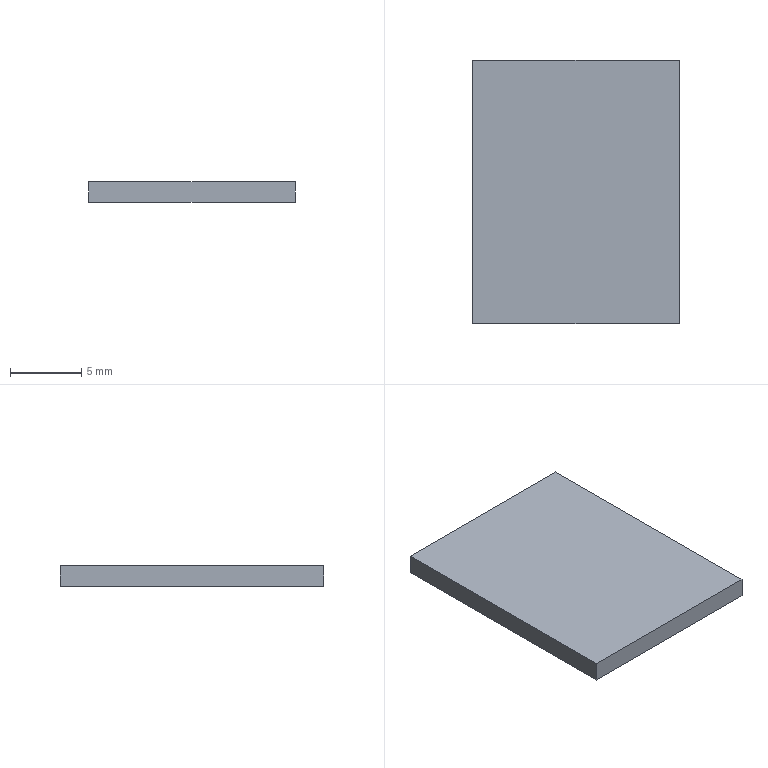Part | Creo | 1 solid | 6 faces | box 14.427 x 18.427 x 1.4 mm | volume 372.198 mm3 | plane 6
STEP:
#1=CARTESIAN_POINT('',(0.,0.,0.));
#2=DIRECTION('',(0.,0.,1.));
#3=DIRECTION('',(1.,0.,0.));
#4=AXIS2_PLACEMENT_3D('',#1,#2,#3);
#5=CARTESIAN_POINT('',(-7.313,-9.113,0.));
#6=VERTEX_POINT('',#5);
#7=CARTESIAN_POINT('',(7.114,-9.113,0.));
#8=VERTEX_POINT('',#7);
#9=CARTESIAN_POINT('',(-7.313,-9.113,0.));
#10=DIRECTION('',(1.,0.,0.));
#11=VECTOR('',#10,14.427);
#12=LINE('',#9,#11);
#13=EDGE_CURVE('',#6,#8,#12,.T.);
#14=ORIENTED_EDGE('',*,*,#13,.T.);
#15=CARTESIAN_POINT('',(7.114,9.314,0.));
#16=VERTEX_POINT('',#15);
#17=CARTESIAN_POINT('',(7.114,-9.113,0.));
#18=DIRECTION('',(0.,1.,0.));
#19=VECTOR('',#18,18.427);
#20=LINE('',#17,#19);
#21=EDGE_CURVE('',#8,#16,#20,.T.);
#22=ORIENTED_EDGE('',*,*,#21,.T.);
#23=CARTESIAN_POINT('',(-7.313,9.314,0.));
#24=VERTEX_POINT('',#23);
#25=CARTESIAN_POINT('',(7.114,9.314,0.));
#26=DIRECTION('',(-1.,0.,0.));
#27=VECTOR('',#26,14.427);
#28=LINE('',#25,#27);
#29=EDGE_CURVE('',#16,#24,#28,.T.);
#30=ORIENTED_EDGE('',*,*,#29,.T.);
#31=CARTESIAN_POINT('',(-7.313,9.314,0.));
#32=DIRECTION('',(0.,-1.,0.));
#33=VECTOR('',#32,18.427);
#34=LINE('',#31,#33);
#35=EDGE_CURVE('',#24,#6,#34,.T.);
#36=ORIENTED_EDGE('',*,*,#35,.T.);
#37=EDGE_LOOP('',(#14,#22,#30,#36));
#38=FACE_OUTER_BOUND('',#37,.F.);
#39=CARTESIAN_POINT('',(0.,0.,0.));
#40=DIRECTION('',(0.,0.,1.));
#41=DIRECTION('',(1.,0.,0.));
#42=AXIS2_PLACEMENT_3D('',#39,#40,#41);
#43=PLANE('',#42);
#44=ADVANCED_FACE('',(#38),#43,.F.);
#45=ORIENTED_EDGE('',*,*,#13,.F.);
#46=CARTESIAN_POINT('',(-7.313,-9.113,1.4));
#47=VERTEX_POINT('',#46);
#48=CARTESIAN_POINT('',(-7.313,-9.113,0.));
#49=DIRECTION('',(0.,0.,1.));
#50=VECTOR('',#49,1.4);
#51=LINE('',#48,#50);
#52=EDGE_CURVE('',#6,#47,#51,.T.);
#53=ORIENTED_EDGE('',*,*,#52,.T.);
#54=CARTESIAN_POINT('',(7.114,-9.113,1.4));
#55=VERTEX_POINT('',#54);
#56=CARTESIAN_POINT('',(-7.313,-9.113,1.4));
#57=DIRECTION('',(1.,0.,0.));
#58=VECTOR('',#57,14.427);
#59=LINE('',#56,#58);
#60=EDGE_CURVE('',#47,#55,#59,.T.);
#61=ORIENTED_EDGE('',*,*,#60,.T.);
#62=CARTESIAN_POINT('',(7.114,-9.113,0.));
#63=DIRECTION('',(0.,0.,1.));
#64=VECTOR('',#63,1.4);
#65=LINE('',#62,#64);
#66=EDGE_CURVE('',#8,#55,#65,.T.);
#67=ORIENTED_EDGE('',*,*,#66,.F.);
#68=EDGE_LOOP('',(#45,#53,#61,#67));
#69=FACE_OUTER_BOUND('',#68,.F.);
#70=CARTESIAN_POINT('',(-7.313,-9.113,0.));
#71=DIRECTION('',(0.,-1.,0.));
#72=DIRECTION('',(1.,0.,0.));
#73=AXIS2_PLACEMENT_3D('',#70,#71,#72);
#74=PLANE('',#73);
#75=ADVANCED_FACE('',(#69),#74,.T.);
#76=ORIENTED_EDGE('',*,*,#35,.F.);
#77=CARTESIAN_POINT('',(-7.313,9.314,1.4));
#78=VERTEX_POINT('',#77);
#79=CARTESIAN_POINT('',(-7.313,9.314,0.));
#80=DIRECTION('',(0.,0.,1.));
#81=VECTOR('',#80,1.4);
#82=LINE('',#79,#81);
#83=EDGE_CURVE('',#24,#78,#82,.T.);
#84=ORIENTED_EDGE('',*,*,#83,.T.);
#85=CARTESIAN_POINT('',(-7.313,9.314,1.4));
#86=DIRECTION('',(0.,-1.,0.));
#87=VECTOR('',#86,18.427);
#88=LINE('',#85,#87);
#89=EDGE_CURVE('',#78,#47,#88,.T.);
#90=ORIENTED_EDGE('',*,*,#89,.T.);
#91=ORIENTED_EDGE('',*,*,#52,.F.);
#92=EDGE_LOOP('',(#76,#84,#90,#91));
#93=FACE_OUTER_BOUND('',#92,.F.);
#94=CARTESIAN_POINT('',(-7.313,9.314,0.));
#95=DIRECTION('',(-1.,0.,0.));
#96=DIRECTION('',(0.,-1.,0.));
#97=AXIS2_PLACEMENT_3D('',#94,#95,#96);
#98=PLANE('',#97);
#99=ADVANCED_FACE('',(#93),#98,.T.);
#100=ORIENTED_EDGE('',*,*,#29,.F.);
#101=CARTESIAN_POINT('',(7.114,9.314,1.4));
#102=VERTEX_POINT('',#101);
#103=CARTESIAN_POINT('',(7.114,9.314,0.));
#104=DIRECTION('',(0.,0.,1.));
#105=VECTOR('',#104,1.4);
#106=LINE('',#103,#105);
#107=EDGE_CURVE('',#16,#102,#106,.T.);
#108=ORIENTED_EDGE('',*,*,#107,.T.);
#109=CARTESIAN_POINT('',(7.114,9.314,1.4));
#110=DIRECTION('',(-1.,0.,0.));
#111=VECTOR('',#110,14.427);
#112=LINE('',#109,#111);
#113=EDGE_CURVE('',#102,#78,#112,.T.);
#114=ORIENTED_EDGE('',*,*,#113,.T.);
#115=ORIENTED_EDGE('',*,*,#83,.F.);
#116=EDGE_LOOP('',(#100,#108,#114,#115));
#117=FACE_OUTER_BOUND('',#116,.F.);
#118=CARTESIAN_POINT('',(7.114,9.314,0.));
#119=DIRECTION('',(0.,1.,0.));
#120=DIRECTION('',(-1.,0.,0.));
#121=AXIS2_PLACEMENT_3D('',#118,#119,#120);
#122=PLANE('',#121);
#123=ADVANCED_FACE('',(#117),#122,.T.);
#124=ORIENTED_EDGE('',*,*,#21,.F.);
#125=ORIENTED_EDGE('',*,*,#66,.T.);
#126=CARTESIAN_POINT('',(7.114,-9.113,1.4));
#127=DIRECTION('',(0.,1.,0.));
#128=VECTOR('',#127,18.427);
#129=LINE('',#126,#128);
#130=EDGE_CURVE('',#55,#102,#129,.T.);
#131=ORIENTED_EDGE('',*,*,#130,.T.);
#132=ORIENTED_EDGE('',*,*,#107,.F.);
#133=EDGE_LOOP('',(#124,#125,#131,#132));
#134=FACE_OUTER_BOUND('',#133,.F.);
#135=CARTESIAN_POINT('',(7.114,-9.113,0.));
#136=DIRECTION('',(1.,0.,0.));
#137=DIRECTION('',(0.,1.,0.));
#138=AXIS2_PLACEMENT_3D('',#135,#136,#137);
#139=PLANE('',#138);
#140=ADVANCED_FACE('',(#134),#139,.T.);
#141=ORIENTED_EDGE('',*,*,#60,.F.);
#142=ORIENTED_EDGE('',*,*,#89,.F.);
#143=ORIENTED_EDGE('',*,*,#113,.F.);
#144=ORIENTED_EDGE('',*,*,#130,.F.);
#145=EDGE_LOOP('',(#141,#142,#143,#144));
#146=FACE_OUTER_BOUND('',#145,.F.);
#147=CARTESIAN_POINT('',(0.,0.,1.4));
#148=DIRECTION('',(0.,0.,1.));
#149=DIRECTION('',(1.,0.,0.));
#150=AXIS2_PLACEMENT_3D('',#147,#148,#149);
#151=PLANE('',#150);
#152=ADVANCED_FACE('',(#146),#151,.T.);
#153=CLOSED_SHELL('',(#44,#75,#99,#123,#140,#152));
#154=MANIFOLD_SOLID_BREP('',#153);
#155=(LENGTH_UNIT()NAMED_UNIT(*)SI_UNIT(.MILLI.,.METRE.));
#156=UNCERTAINTY_MEASURE_WITH_UNIT(LENGTH_MEASURE(0.002344),#155,'','');
#157=(NAMED_UNIT(*)PLANE_ANGLE_UNIT()SI_UNIT($,.RADIAN.));
#158=PLANE_ANGLE_MEASURE_WITH_UNIT(PLANE_ANGLE_MEASURE(0.01745),#157);
#159=(CONVERSION_BASED_UNIT('DEGREE',#158)NAMED_UNIT(*)PLANE_ANGLE_UNIT());
#160=(NAMED_UNIT(*)SI_UNIT($,.STERADIAN.)SOLID_ANGLE_UNIT());
#161=(GEOMETRIC_REPRESENTATION_CONTEXT(3)GLOBAL_UNCERTAINTY_ASSIGNED_CONTEXT((#156))GLOBAL_UNIT_ASSIGNED_CONTEXT((#155,#159,#160))REPRESENTATION_CONTEXT('',''));
#162=ADVANCED_BREP_SHAPE_REPRESENTATION('',(#4,#154),#161);